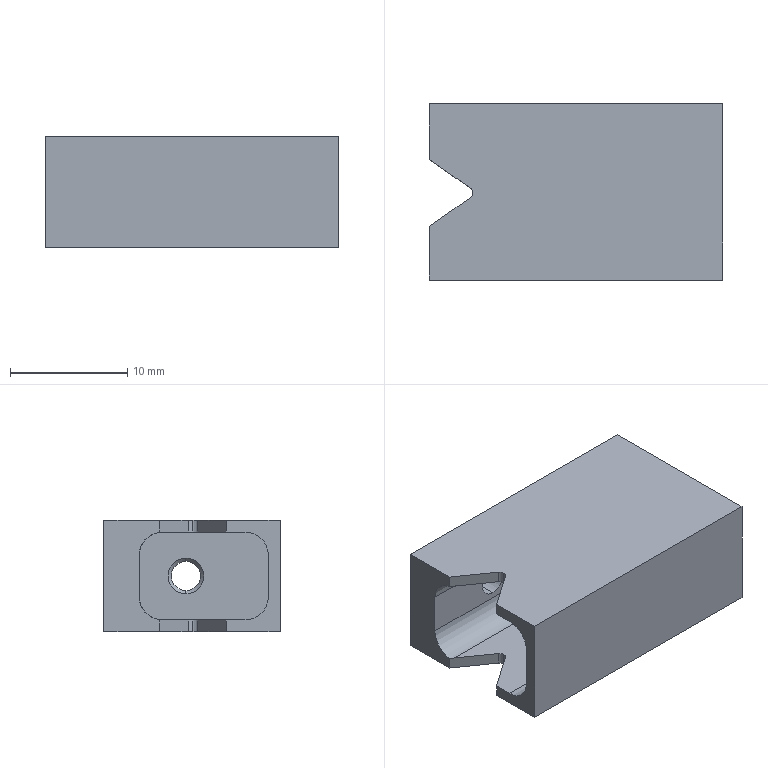Part | SolidWorks | features BaseBody 1 | 1 solid | 32 faces | box 25 x 15.037 x 9.5 mm | volume 1907 mm3 | plane 16 | cylinder 14 | cone 2 | commonest cylinder face diameters 2.5 x6 1 x4 4 x4
STEP:
#1=CARTESIAN_POINT('',(-21.301,7.437,8.5));
#2=VERTEX_POINT('',#1);
#3=CARTESIAN_POINT('',(-21.514,7.847,8.5));
#4=VERTEX_POINT('',#3);
#5=CARTESIAN_POINT('',(-21.801,7.437,8.5));
#6=DIRECTION('',(0.,0.,1.));
#7=DIRECTION('',(1.,0.,0.));
#8=AXIS2_PLACEMENT_3D('',#5,#6,#7);
#9=CIRCLE('',#8,0.5);
#10=EDGE_CURVE('',#2,#4,#9,.T.);
#11=ORIENTED_EDGE('',*,*,#10,.F.);
#12=CARTESIAN_POINT('',(-21.301,7.437,9.5));
#13=VERTEX_POINT('',#12);
#14=CARTESIAN_POINT('',(-21.301,7.437,9.5));
#15=DIRECTION('',(0.,0.,1.));
#16=VECTOR('',#15,1000.);
#17=LINE('',#14,#16);
#18=EDGE_CURVE('',#2,#13,#17,.T.);
#19=ORIENTED_EDGE('',*,*,#18,.T.);
#20=CARTESIAN_POINT('',(-21.514,7.847,9.5));
#21=VERTEX_POINT('',#20);
#22=CARTESIAN_POINT('',(-21.801,7.437,9.5));
#23=DIRECTION('',(0.,0.,1.));
#24=DIRECTION('',(1.,0.,0.));
#25=AXIS2_PLACEMENT_3D('',#22,#23,#24);
#26=CIRCLE('',#25,0.5);
#27=EDGE_CURVE('',#13,#21,#26,.T.);
#28=ORIENTED_EDGE('',*,*,#27,.T.);
#29=CARTESIAN_POINT('',(-21.514,7.847,9.5));
#30=DIRECTION('',(0.,0.,-1.));
#31=VECTOR('',#30,1000.);
#32=LINE('',#29,#31);
#33=EDGE_CURVE('',#21,#4,#32,.T.);
#34=ORIENTED_EDGE('',*,*,#33,.T.);
#35=EDGE_LOOP('',(#11,#19,#28,#34));
#36=FACE_OUTER_BOUND('',#35,.T.);
#37=CARTESIAN_POINT('',(-21.801,7.437,9.5));
#38=DIRECTION('',(0.,0.,1.));
#39=DIRECTION('',(1.,0.,0.));
#40=AXIS2_PLACEMENT_3D('',#37,#38,#39);
#41=CYLINDRICAL_SURFACE('',#40,0.5);
#42=ADVANCED_FACE('',(#36),#41,.F.);
#43=CARTESIAN_POINT('',(0.,8.037,6.));
#44=VERTEX_POINT('',#43);
#45=CARTESIAN_POINT('',(0.,8.037,3.5));
#46=VERTEX_POINT('',#45);
#47=CARTESIAN_POINT('',(0.,8.037,4.75));
#48=DIRECTION('',(1.,0.,0.));
#49=DIRECTION('',(0.,0.,1.));
#50=AXIS2_PLACEMENT_3D('',#47,#48,#49);
#51=CIRCLE('',#50,1.25);
#52=EDGE_CURVE('',#44,#46,#51,.T.);
#53=ORIENTED_EDGE('',*,*,#52,.T.);
#54=CARTESIAN_POINT('',(-4.725,8.037,3.5));
#55=VERTEX_POINT('',#54);
#56=CARTESIAN_POINT('',(-5.,8.037,3.5));
#57=DIRECTION('',(-1.,0.,0.));
#58=VECTOR('',#57,1000.);
#59=LINE('',#56,#58);
#60=EDGE_CURVE('',#46,#55,#59,.T.);
#61=ORIENTED_EDGE('',*,*,#60,.T.);
#62=CARTESIAN_POINT('',(-4.725,8.037,6.));
#63=VERTEX_POINT('',#62);
#64=CARTESIAN_POINT('',(-4.725,8.037,4.75));
#65=DIRECTION('',(1.,0.,0.));
#66=DIRECTION('',(0.,0.,1.));
#67=AXIS2_PLACEMENT_3D('',#64,#65,#66);
#68=CIRCLE('',#67,1.25);
#69=EDGE_CURVE('',#63,#55,#68,.T.);
#70=ORIENTED_EDGE('',*,*,#69,.F.);
#71=CARTESIAN_POINT('',(-5.,8.037,6.));
#72=DIRECTION('',(-1.,0.,0.));
#73=VECTOR('',#72,1000.);
#74=LINE('',#71,#73);
#75=EDGE_CURVE('',#44,#63,#74,.T.);
#76=ORIENTED_EDGE('',*,*,#75,.F.);
#77=EDGE_LOOP('',(#53,#61,#70,#76));
#78=FACE_OUTER_BOUND('',#77,.T.);
#79=CARTESIAN_POINT('',(-5.,8.037,4.75));
#80=DIRECTION('',(-1.,0.,0.));
#81=DIRECTION('',(0.,0.,1.));
#82=AXIS2_PLACEMENT_3D('',#79,#80,#81);
#83=CYLINDRICAL_SURFACE('',#82,1.25);
#84=ADVANCED_FACE('',(#78),#83,.F.);
#85=CARTESIAN_POINT('',(-18.,12.037,6.));
#86=VERTEX_POINT('',#85);
#87=CARTESIAN_POINT('',(-18.,12.037,3.5));
#88=VERTEX_POINT('',#87);
#89=CARTESIAN_POINT('',(-18.,12.037,4.75));
#90=DIRECTION('',(0.,-1.,0.));
#91=DIRECTION('',(0.,0.,1.));
#92=AXIS2_PLACEMENT_3D('',#89,#90,#91);
#93=CIRCLE('',#92,1.25);
#94=EDGE_CURVE('',#86,#88,#93,.T.);
#95=ORIENTED_EDGE('',*,*,#94,.T.);
#96=CARTESIAN_POINT('',(-18.,15.037,3.5));
#97=VERTEX_POINT('',#96);
#98=CARTESIAN_POINT('',(-18.,15.037,3.5));
#99=DIRECTION('',(0.,1.,0.));
#100=VECTOR('',#99,1000.);
#101=LINE('',#98,#100);
#102=EDGE_CURVE('',#88,#97,#101,.T.);
#103=ORIENTED_EDGE('',*,*,#102,.T.);
#104=CARTESIAN_POINT('',(-18.,15.037,6.));
#105=VERTEX_POINT('',#104);
#106=CARTESIAN_POINT('',(-18.,15.037,4.75));
#107=DIRECTION('',(0.,1.,0.));
#108=DIRECTION('',(0.,0.,1.));
#109=AXIS2_PLACEMENT_3D('',#106,#107,#108);
#110=CIRCLE('',#109,1.25);
#111=EDGE_CURVE('',#97,#105,#110,.T.);
#112=ORIENTED_EDGE('',*,*,#111,.T.);
#113=CARTESIAN_POINT('',(-18.,15.037,6.));
#114=DIRECTION('',(0.,1.,0.));
#115=VECTOR('',#114,1000.);
#116=LINE('',#113,#115);
#117=EDGE_CURVE('',#86,#105,#116,.T.);
#118=ORIENTED_EDGE('',*,*,#117,.F.);
#119=EDGE_LOOP('',(#95,#103,#112,#118));
#120=FACE_OUTER_BOUND('',#119,.T.);
#121=CARTESIAN_POINT('',(-18.,15.037,4.75));
#122=DIRECTION('',(0.,1.,0.));
#123=DIRECTION('',(0.,0.,1.));
#124=AXIS2_PLACEMENT_3D('',#121,#122,#123);
#125=CYLINDRICAL_SURFACE('',#124,1.25);
#126=ADVANCED_FACE('',(#120),#125,.F.);
#127=CARTESIAN_POINT('',(-8.,12.037,6.));
#128=VERTEX_POINT('',#127);
#129=CARTESIAN_POINT('',(-8.,12.037,3.5));
#130=VERTEX_POINT('',#129);
#131=CARTESIAN_POINT('',(-8.,12.037,4.75));
#132=DIRECTION('',(0.,-1.,0.));
#133=DIRECTION('',(0.,0.,1.));
#134=AXIS2_PLACEMENT_3D('',#131,#132,#133);
#135=CIRCLE('',#134,1.25);
#136=EDGE_CURVE('',#128,#130,#135,.T.);
#137=ORIENTED_EDGE('',*,*,#136,.T.);
#138=CARTESIAN_POINT('',(-8.,15.037,3.5));
#139=VERTEX_POINT('',#138);
#140=CARTESIAN_POINT('',(-8.,15.037,3.5));
#141=DIRECTION('',(0.,1.,0.));
#142=VECTOR('',#141,1000.);
#143=LINE('',#140,#142);
#144=EDGE_CURVE('',#130,#139,#143,.T.);
#145=ORIENTED_EDGE('',*,*,#144,.T.);
#146=CARTESIAN_POINT('',(-8.,15.037,6.));
#147=VERTEX_POINT('',#146);
#148=CARTESIAN_POINT('',(-8.,15.037,4.75));
#149=DIRECTION('',(0.,1.,0.));
#150=DIRECTION('',(0.,0.,1.));
#151=AXIS2_PLACEMENT_3D('',#148,#149,#150);
#152=CIRCLE('',#151,1.25);
#153=EDGE_CURVE('',#139,#147,#152,.T.);
#154=ORIENTED_EDGE('',*,*,#153,.T.);
#155=CARTESIAN_POINT('',(-8.,15.037,6.));
#156=DIRECTION('',(0.,1.,0.));
#157=VECTOR('',#156,1000.);
#158=LINE('',#155,#157);
#159=EDGE_CURVE('',#128,#147,#158,.T.);
#160=ORIENTED_EDGE('',*,*,#159,.F.);
#161=EDGE_LOOP('',(#137,#145,#154,#160));
#162=FACE_OUTER_BOUND('',#161,.T.);
#163=CARTESIAN_POINT('',(-8.,15.037,4.75));
#164=DIRECTION('',(0.,1.,0.));
#165=DIRECTION('',(0.,0.,1.));
#166=AXIS2_PLACEMENT_3D('',#163,#164,#165);
#167=CYLINDRICAL_SURFACE('',#166,1.25);
#168=ADVANCED_FACE('',(#162),#167,.F.);
#169=CARTESIAN_POINT('',(-21.301,7.437,0.));
#170=VERTEX_POINT('',#169);
#171=CARTESIAN_POINT('',(-21.514,7.847,0.));
#172=VERTEX_POINT('',#171);
#173=CARTESIAN_POINT('',(-21.801,7.437,0.));
#174=DIRECTION('',(0.,0.,1.));
#175=DIRECTION('',(1.,0.,0.));
#176=AXIS2_PLACEMENT_3D('',#173,#174,#175);
#177=CIRCLE('',#176,0.5);
#178=EDGE_CURVE('',#170,#172,#177,.T.);
#179=ORIENTED_EDGE('',*,*,#178,.F.);
#180=CARTESIAN_POINT('',(-21.301,7.437,1.));
#181=VERTEX_POINT('',#180);
#182=CARTESIAN_POINT('',(-21.301,7.437,9.5));
#183=DIRECTION('',(0.,0.,1.));
#184=VECTOR('',#183,1000.);
#185=LINE('',#182,#184);
#186=EDGE_CURVE('',#170,#181,#185,.T.);
#187=ORIENTED_EDGE('',*,*,#186,.T.);
#188=CARTESIAN_POINT('',(-21.514,7.847,1.));
#189=VERTEX_POINT('',#188);
#190=CARTESIAN_POINT('',(-21.801,7.437,1.));
#191=DIRECTION('',(0.,0.,1.));
#192=DIRECTION('',(1.,0.,0.));
#193=AXIS2_PLACEMENT_3D('',#190,#191,#192);
#194=CIRCLE('',#193,0.5);
#195=EDGE_CURVE('',#181,#189,#194,.T.);
#196=ORIENTED_EDGE('',*,*,#195,.T.);
#197=CARTESIAN_POINT('',(-21.514,7.847,9.5));
#198=DIRECTION('',(0.,0.,-1.));
#199=VECTOR('',#198,1000.);
#200=LINE('',#197,#199);
#201=EDGE_CURVE('',#189,#172,#200,.T.);
#202=ORIENTED_EDGE('',*,*,#201,.T.);
#203=EDGE_LOOP('',(#179,#187,#196,#202));
#204=FACE_OUTER_BOUND('',#203,.T.);
#205=CARTESIAN_POINT('',(-21.801,7.437,9.5));
#206=DIRECTION('',(0.,0.,1.));
#207=DIRECTION('',(1.,0.,0.));
#208=AXIS2_PLACEMENT_3D('',#205,#206,#207);
#209=CYLINDRICAL_SURFACE('',#208,0.5);
#210=ADVANCED_FACE('',(#204),#209,.F.);
#211=ORIENTED_EDGE('',*,*,#69,.T.);
#212=CARTESIAN_POINT('',(-5.,8.037,3.225));
#213=VERTEX_POINT('',#212);
#214=CARTESIAN_POINT('',(-5.,8.037,3.225));
#215=DIRECTION('',(-0.7071,0.,-0.7071));
#216=VECTOR('',#215,1000.);
#217=LINE('',#214,#216);
#218=EDGE_CURVE('',#55,#213,#217,.T.);
#219=ORIENTED_EDGE('',*,*,#218,.T.);
#220=CARTESIAN_POINT('',(-5.,8.037,6.275));
#221=VERTEX_POINT('',#220);
#222=CARTESIAN_POINT('',(-5.,8.037,4.75));
#223=DIRECTION('',(1.,0.,0.));
#224=DIRECTION('',(0.,0.,1.));
#225=AXIS2_PLACEMENT_3D('',#222,#223,#224);
#226=CIRCLE('',#225,1.525);
#227=EDGE_CURVE('',#221,#213,#226,.T.);
#228=ORIENTED_EDGE('',*,*,#227,.F.);
#229=CARTESIAN_POINT('',(-5.,8.037,6.275));
#230=DIRECTION('',(-0.7071,0.,0.7071));
#231=VECTOR('',#230,1000.);
#232=LINE('',#229,#231);
#233=EDGE_CURVE('',#63,#221,#232,.T.);
#234=ORIENTED_EDGE('',*,*,#233,.F.);
#235=EDGE_LOOP('',(#211,#219,#228,#234));
#236=FACE_OUTER_BOUND('',#235,.T.);
#237=CARTESIAN_POINT('',(-5.,8.037,4.75));
#238=DIRECTION('',(-1.,0.,0.));
#239=DIRECTION('',(0.,0.,1.));
#240=AXIS2_PLACEMENT_3D('',#237,#238,#239);
#241=CONICAL_SURFACE('',#240,1.525,0.7854);
#242=ADVANCED_FACE('',(#236),#241,.F.);
#243=CARTESIAN_POINT('',(-25.,10.288,9.5));
#244=VERTEX_POINT('',#243);
#245=CARTESIAN_POINT('',(-21.514,7.847,9.5));
#246=DIRECTION('',(-0.8192,0.5736,0.));
#247=VECTOR('',#246,1000.);
#248=LINE('',#245,#247);
#249=EDGE_CURVE('',#21,#244,#248,.T.);
#250=ORIENTED_EDGE('',*,*,#249,.F.);
#251=ORIENTED_EDGE('',*,*,#27,.F.);
#252=CARTESIAN_POINT('',(-21.514,7.028,9.5));
#253=VERTEX_POINT('',#252);
#254=CARTESIAN_POINT('',(-21.801,7.437,9.5));
#255=DIRECTION('',(0.,0.,1.));
#256=DIRECTION('',(1.,0.,0.));
#257=AXIS2_PLACEMENT_3D('',#254,#255,#256);
#258=CIRCLE('',#257,0.5);
#259=EDGE_CURVE('',#253,#13,#258,.T.);
#260=ORIENTED_EDGE('',*,*,#259,.F.);
#261=CARTESIAN_POINT('',(-25.,4.587,9.5));
#262=VERTEX_POINT('',#261);
#263=CARTESIAN_POINT('',(-25.,4.587,9.5));
#264=DIRECTION('',(0.8192,0.5736,0.));
#265=VECTOR('',#264,1000.);
#266=LINE('',#263,#265);
#267=EDGE_CURVE('',#262,#253,#266,.T.);
#268=ORIENTED_EDGE('',*,*,#267,.F.);
#269=CARTESIAN_POINT('',(-25.,0.,9.5));
#270=VERTEX_POINT('',#269);
#271=CARTESIAN_POINT('',(-25.,0.,9.5));
#272=DIRECTION('',(0.,1.,0.));
#273=VECTOR('',#272,1000.);
#274=LINE('',#271,#273);
#275=EDGE_CURVE('',#270,#262,#274,.T.);
#276=ORIENTED_EDGE('',*,*,#275,.F.);
#277=CARTESIAN_POINT('',(0.,0.,9.5));
#278=VERTEX_POINT('',#277);
#279=CARTESIAN_POINT('',(0.,0.,9.5));
#280=DIRECTION('',(-1.,0.,0.));
#281=VECTOR('',#280,1000.);
#282=LINE('',#279,#281);
#283=EDGE_CURVE('',#278,#270,#282,.T.);
#284=ORIENTED_EDGE('',*,*,#283,.F.);
#285=CARTESIAN_POINT('',(0.,15.037,9.5));
#286=VERTEX_POINT('',#285);
#287=CARTESIAN_POINT('',(0.,0.,9.5));
#288=DIRECTION('',(0.,-1.,0.));
#289=VECTOR('',#288,1000.);
#290=LINE('',#287,#289);
#291=EDGE_CURVE('',#286,#278,#290,.T.);
#292=ORIENTED_EDGE('',*,*,#291,.F.);
#293=CARTESIAN_POINT('',(-25.,15.037,9.5));
#294=VERTEX_POINT('',#293);
#295=CARTESIAN_POINT('',(0.,15.037,9.5));
#296=DIRECTION('',(1.,0.,0.));
#297=VECTOR('',#296,1000.);
#298=LINE('',#295,#297);
#299=EDGE_CURVE('',#294,#286,#298,.T.);
#300=ORIENTED_EDGE('',*,*,#299,.F.);
#301=CARTESIAN_POINT('',(-25.,0.,9.5));
#302=DIRECTION('',(0.,1.,0.));
#303=VECTOR('',#302,1000.);
#304=LINE('',#301,#303);
#305=EDGE_CURVE('',#244,#294,#304,.T.);
#306=ORIENTED_EDGE('',*,*,#305,.F.);
#307=EDGE_LOOP('',(#250,#251,#260,#268,#276,#284,#292,#300,#306));
#308=FACE_OUTER_BOUND('',#307,.T.);
#309=CARTESIAN_POINT('',(0.,0.,9.5));
#310=DIRECTION('',(0.,0.,-1.));
#311=DIRECTION('',(-1.,0.,0.));
#312=AXIS2_PLACEMENT_3D('',#309,#310,#311);
#313=PLANE('',#312);
#314=ADVANCED_FACE('',(#308),#313,.F.);
#315=CARTESIAN_POINT('',(-25.,12.037,3.));
#316=VERTEX_POINT('',#315);
#317=CARTESIAN_POINT('',(-25.,10.288,1.016));
#318=VERTEX_POINT('',#317);
#319=CARTESIAN_POINT('',(-25.,10.037,3.));
#320=DIRECTION('',(-1.,0.,0.));
#321=DIRECTION('',(0.,0.,-1.));
#322=AXIS2_PLACEMENT_3D('',#319,#320,#321);
#323=CIRCLE('',#322,2.);
#324=EDGE_CURVE('',#316,#318,#323,.T.);
#325=ORIENTED_EDGE('',*,*,#324,.F.);
#326=CARTESIAN_POINT('',(-25.,12.037,6.5));
#327=VERTEX_POINT('',#326);
#328=CARTESIAN_POINT('',(-25.,12.037,9.5));
#329=DIRECTION('',(0.,0.,-1.));
#330=VECTOR('',#329,1000.);
#331=LINE('',#328,#330);
#332=EDGE_CURVE('',#327,#316,#331,.T.);
#333=ORIENTED_EDGE('',*,*,#332,.F.);
#334=CARTESIAN_POINT('',(-25.,10.288,8.484));
#335=VERTEX_POINT('',#334);
#336=CARTESIAN_POINT('',(-25.,10.037,6.5));
#337=DIRECTION('',(-1.,0.,0.));
#338=DIRECTION('',(0.,0.,-1.));
#339=AXIS2_PLACEMENT_3D('',#336,#337,#338);
#340=CIRCLE('',#339,2.);
#341=EDGE_CURVE('',#335,#327,#340,.T.);
#342=ORIENTED_EDGE('',*,*,#341,.F.);
#343=CARTESIAN_POINT('',(-25.,10.288,9.5));
#344=DIRECTION('',(0.,0.,-1.));
#345=VECTOR('',#344,1000.);
#346=LINE('',#343,#345);
#347=EDGE_CURVE('',#244,#335,#346,.T.);
#348=ORIENTED_EDGE('',*,*,#347,.F.);
#349=ORIENTED_EDGE('',*,*,#305,.T.);
#350=CARTESIAN_POINT('',(-25.,15.037,0.));
#351=VERTEX_POINT('',#350);
#352=CARTESIAN_POINT('',(-25.,15.037,9.5));
#353=DIRECTION('',(0.,0.,1.));
#354=VECTOR('',#353,1000.);
#355=LINE('',#352,#354);
#356=EDGE_CURVE('',#351,#294,#355,.T.);
#357=ORIENTED_EDGE('',*,*,#356,.F.);
#358=CARTESIAN_POINT('',(-25.,10.288,0.));
#359=VERTEX_POINT('',#358);
#360=CARTESIAN_POINT('',(-25.,10.288,0.));
#361=DIRECTION('',(0.,1.,0.));
#362=VECTOR('',#361,1000.);
#363=LINE('',#360,#362);
#364=EDGE_CURVE('',#359,#351,#363,.T.);
#365=ORIENTED_EDGE('',*,*,#364,.F.);
#366=CARTESIAN_POINT('',(-25.,10.288,9.5));
#367=DIRECTION('',(0.,0.,1.));
#368=VECTOR('',#367,1000.);
#369=LINE('',#366,#368);
#370=EDGE_CURVE('',#359,#318,#369,.T.);
#371=ORIENTED_EDGE('',*,*,#370,.T.);
#372=EDGE_LOOP('',(#325,#333,#342,#348,#349,#357,#365,#371));
#373=FACE_OUTER_BOUND('',#372,.T.);
#374=CARTESIAN_POINT('',(-25.,10.288,9.5));
#375=DIRECTION('',(1.,0.,0.));
#376=DIRECTION('',(0.,0.,-1.));
#377=AXIS2_PLACEMENT_3D('',#374,#375,#376);
#378=PLANE('',#377);
#379=ADVANCED_FACE('',(#373),#378,.F.);
#380=CARTESIAN_POINT('',(-24.642,10.037,8.5));
#381=VERTEX_POINT('',#380);
#382=CARTESIAN_POINT('',(-24.642,10.037,8.5));
#383=CARTESIAN_POINT('',(-24.762,10.121,8.5));
#384=CARTESIAN_POINT('',(-24.881,10.205,8.495));
#385=CARTESIAN_POINT('',(-25.,10.288,8.484));
#386=(BOUNDED_CURVE()B_SPLINE_CURVE(3,(#382,#383,#384,#385),.UNSPECIFIED.,.F.,.F.)B_SPLINE_CURVE_WITH_KNOTS((4,4),(1.571,1.696),.UNSPECIFIED.)CURVE()GEOMETRIC_REPRESENTATION_ITEM()RATIONAL_B_SPLINE_CURVE((1.,0.9987,0.9987,1.))REPRESENTATION_ITEM(''));
#387=EDGE_CURVE('',#381,#335,#386,.T.);
#388=ORIENTED_EDGE('',*,*,#387,.F.);
#389=CARTESIAN_POINT('',(-25.,10.288,8.5));
#390=DIRECTION('',(-0.8192,0.5736,0.));
#391=VECTOR('',#390,1000.);
#392=LINE('',#389,#391);
#393=EDGE_CURVE('',#4,#381,#392,.T.);
#394=ORIENTED_EDGE('',*,*,#393,.F.);
#395=ORIENTED_EDGE('',*,*,#33,.F.);
#396=ORIENTED_EDGE('',*,*,#249,.T.);
#397=ORIENTED_EDGE('',*,*,#347,.T.);
#398=EDGE_LOOP('',(#388,#394,#395,#396,#397));
#399=FACE_OUTER_BOUND('',#398,.T.);
#400=CARTESIAN_POINT('',(-25.,10.288,9.5));
#401=DIRECTION('',(0.5736,0.8192,0.));
#402=DIRECTION('',(-0.8192,0.5736,0.));
#403=AXIS2_PLACEMENT_3D('',#400,#401,#402);
#404=PLANE('',#403);
#405=ADVANCED_FACE('',(#399),#404,.F.);
#406=ORIENTED_EDGE('',*,*,#18,.F.);
#407=CARTESIAN_POINT('',(-21.514,7.028,8.5));
#408=VERTEX_POINT('',#407);
#409=CARTESIAN_POINT('',(-21.801,7.437,8.5));
#410=DIRECTION('',(0.,0.,1.));
#411=DIRECTION('',(1.,0.,0.));
#412=AXIS2_PLACEMENT_3D('',#409,#410,#411);
#413=CIRCLE('',#412,0.5);
#414=EDGE_CURVE('',#408,#2,#413,.T.);
#415=ORIENTED_EDGE('',*,*,#414,.F.);
#416=CARTESIAN_POINT('',(-21.514,7.028,9.5));
#417=DIRECTION('',(0.,0.,-1.));
#418=VECTOR('',#417,1000.);
#419=LINE('',#416,#418);
#420=EDGE_CURVE('',#253,#408,#419,.T.);
#421=ORIENTED_EDGE('',*,*,#420,.F.);
#422=ORIENTED_EDGE('',*,*,#259,.T.);
#423=EDGE_LOOP('',(#406,#415,#421,#422));
#424=FACE_OUTER_BOUND('',#423,.T.);
#425=CARTESIAN_POINT('',(-21.801,7.437,9.5));
#426=DIRECTION('',(0.,0.,1.));
#427=DIRECTION('',(1.,0.,0.));
#428=AXIS2_PLACEMENT_3D('',#425,#426,#427);
#429=CYLINDRICAL_SURFACE('',#428,0.5);
#430=ADVANCED_FACE('',(#424),#429,.F.);
#431=ORIENTED_EDGE('',*,*,#420,.T.);
#432=CARTESIAN_POINT('',(-25.,4.587,8.5));
#433=VERTEX_POINT('',#432);
#434=CARTESIAN_POINT('',(-20.929,7.437,8.5));
#435=DIRECTION('',(0.8192,0.5736,0.));
#436=VECTOR('',#435,1000.);
#437=LINE('',#434,#436);
#438=EDGE_CURVE('',#433,#408,#437,.T.);
#439=ORIENTED_EDGE('',*,*,#438,.F.);
#440=CARTESIAN_POINT('',(-25.,4.587,9.5));
#441=DIRECTION('',(0.,0.,-1.));
#442=VECTOR('',#441,1000.);
#443=LINE('',#440,#442);
#444=EDGE_CURVE('',#262,#433,#443,.T.);
#445=ORIENTED_EDGE('',*,*,#444,.F.);
#446=ORIENTED_EDGE('',*,*,#267,.T.);
#447=EDGE_LOOP('',(#431,#439,#445,#446));
#448=FACE_OUTER_BOUND('',#447,.T.);
#449=CARTESIAN_POINT('',(-20.929,7.437,9.5));
#450=DIRECTION('',(0.5736,-0.8192,0.));
#451=DIRECTION('',(0.8192,0.5736,0.));
#452=AXIS2_PLACEMENT_3D('',#449,#450,#451);
#453=PLANE('',#452);
#454=ADVANCED_FACE('',(#448),#453,.F.);
#455=CARTESIAN_POINT('',(-25.,3.,1.));
#456=VERTEX_POINT('',#455);
#457=CARTESIAN_POINT('',(-25.,1.,3.));
#458=VERTEX_POINT('',#457);
#459=CARTESIAN_POINT('',(-25.,3.,3.));
#460=DIRECTION('',(-1.,0.,0.));
#461=DIRECTION('',(0.,0.,-1.));
#462=AXIS2_PLACEMENT_3D('',#459,#460,#461);
#463=CIRCLE('',#462,2.);
#464=EDGE_CURVE('',#456,#458,#463,.T.);
#465=ORIENTED_EDGE('',*,*,#464,.F.);
#466=CARTESIAN_POINT('',(-25.,4.587,1.));
#467=VERTEX_POINT('',#466);
#468=CARTESIAN_POINT('',(-25.,12.037,1.));
#469=DIRECTION('',(0.,1.,0.));
#470=VECTOR('',#469,1000.);
#471=LINE('',#468,#470);
#472=EDGE_CURVE('',#456,#467,#471,.T.);
#473=ORIENTED_EDGE('',*,*,#472,.T.);
#474=CARTESIAN_POINT('',(-25.,4.587,0.));
#475=VERTEX_POINT('',#474);
#476=CARTESIAN_POINT('',(-25.,4.587,9.5));
#477=DIRECTION('',(0.,0.,-1.));
#478=VECTOR('',#477,1000.);
#479=LINE('',#476,#478);
#480=EDGE_CURVE('',#467,#475,#479,.T.);
#481=ORIENTED_EDGE('',*,*,#480,.T.);
#482=CARTESIAN_POINT('',(-25.,0.,0.));
#483=VERTEX_POINT('',#482);
#484=CARTESIAN_POINT('',(-25.,4.587,0.));
#485=DIRECTION('',(0.,1.,0.));
#486=VECTOR('',#485,1000.);
#487=LINE('',#484,#486);
#488=EDGE_CURVE('',#483,#475,#487,.T.);
#489=ORIENTED_EDGE('',*,*,#488,.F.);
#490=CARTESIAN_POINT('',(-25.,0.,9.5));
#491=DIRECTION('',(0.,0.,-1.));
#492=VECTOR('',#491,1000.);
#493=LINE('',#490,#492);
#494=EDGE_CURVE('',#270,#483,#493,.T.);
#495=ORIENTED_EDGE('',*,*,#494,.F.);
#496=ORIENTED_EDGE('',*,*,#275,.T.);
#497=ORIENTED_EDGE('',*,*,#444,.T.);
#498=CARTESIAN_POINT('',(-25.,3.,8.5));
#499=VERTEX_POINT('',#498);
#500=CARTESIAN_POINT('',(-25.,4.587,8.5));
#501=DIRECTION('',(0.,1.,0.));
#502=VECTOR('',#501,1000.);
#503=LINE('',#500,#502);
#504=EDGE_CURVE('',#499,#433,#503,.T.);
#505=ORIENTED_EDGE('',*,*,#504,.F.);
#506=CARTESIAN_POINT('',(-25.,1.,6.5));
#507=VERTEX_POINT('',#506);
#508=CARTESIAN_POINT('',(-25.,3.,6.5));
#509=DIRECTION('',(-1.,0.,0.));
#510=DIRECTION('',(0.,0.,-1.));
#511=AXIS2_PLACEMENT_3D('',#508,#509,#510);
#512=CIRCLE('',#511,2.);
#513=EDGE_CURVE('',#507,#499,#512,.T.);
#514=ORIENTED_EDGE('',*,*,#513,.F.);
#515=CARTESIAN_POINT('',(-25.,1.,9.5));
#516=DIRECTION('',(0.,0.,1.));
#517=VECTOR('',#516,1000.);
#518=LINE('',#515,#517);
#519=EDGE_CURVE('',#458,#507,#518,.T.);
#520=ORIENTED_EDGE('',*,*,#519,.F.);
#521=EDGE_LOOP('',(#465,#473,#481,#489,#495,#496,#497,#505,#514,#520));
#522=FACE_OUTER_BOUND('',#521,.T.);
#523=CARTESIAN_POINT('',(-25.,4.587,9.5));
#524=DIRECTION('',(1.,0.,0.));
#525=DIRECTION('',(0.,0.,-1.));
#526=AXIS2_PLACEMENT_3D('',#523,#524,#525);
#527=PLANE('',#526);
#528=ADVANCED_FACE('',(#522),#527,.F.);
#529=CARTESIAN_POINT('',(0.,0.,0.));
#530=VERTEX_POINT('',#529);
#531=CARTESIAN_POINT('',(0.,0.,9.5));
#532=DIRECTION('',(0.,0.,-1.));
#533=VECTOR('',#532,1000.);
#534=LINE('',#531,#533);
#535=EDGE_CURVE('',#278,#530,#534,.T.);
#536=ORIENTED_EDGE('',*,*,#535,.F.);
#537=ORIENTED_EDGE('',*,*,#283,.T.);
#538=ORIENTED_EDGE('',*,*,#494,.T.);
#539=CARTESIAN_POINT('',(-25.,0.,0.));
#540=DIRECTION('',(-1.,0.,0.));
#541=VECTOR('',#540,1000.);
#542=LINE('',#539,#541);
#543=EDGE_CURVE('',#530,#483,#542,.T.);
#544=ORIENTED_EDGE('',*,*,#543,.F.);
#545=EDGE_LOOP('',(#536,#537,#538,#544));
#546=FACE_OUTER_BOUND('',#545,.T.);
#547=CARTESIAN_POINT('',(-25.,0.,9.5));
#548=DIRECTION('',(0.,1.,0.));
#549=DIRECTION('',(0.,0.,1.));
#550=AXIS2_PLACEMENT_3D('',#547,#548,#549);
#551=PLANE('',#550);
#552=ADVANCED_FACE('',(#546),#551,.F.);
#553=CARTESIAN_POINT('',(0.,15.037,0.));
#554=VERTEX_POINT('',#553);
#555=CARTESIAN_POINT('',(0.,15.037,9.5));
#556=DIRECTION('',(0.,0.,-1.));
#557=VECTOR('',#556,1000.);
#558=LINE('',#555,#557);
#559=EDGE_CURVE('',#286,#554,#558,.T.);
#560=ORIENTED_EDGE('',*,*,#559,.F.);
#561=ORIENTED_EDGE('',*,*,#291,.T.);
#562=ORIENTED_EDGE('',*,*,#535,.T.);
#563=CARTESIAN_POINT('',(0.,15.037,0.));
#564=DIRECTION('',(0.,-1.,0.));
#565=VECTOR('',#564,1000.);
#566=LINE('',#563,#565);
#567=EDGE_CURVE('',#554,#530,#566,.T.);
#568=ORIENTED_EDGE('',*,*,#567,.F.);
#569=EDGE_LOOP('',(#560,#561,#562,#568));
#570=FACE_OUTER_BOUND('',#569,.T.);
#571=ORIENTED_EDGE('',*,*,#52,.F.);
#572=CARTESIAN_POINT('',(0.,8.037,4.75));
#573=DIRECTION('',(1.,0.,0.));
#574=DIRECTION('',(0.,0.,1.));
#575=AXIS2_PLACEMENT_3D('',#572,#573,#574);
#576=CIRCLE('',#575,1.25);
#577=EDGE_CURVE('',#46,#44,#576,.T.);
#578=ORIENTED_EDGE('',*,*,#577,.F.);
#579=EDGE_LOOP('',(#571,#578));
#580=FACE_BOUND('',#579,.T.);
#581=CARTESIAN_POINT('',(0.,15.037,9.5));
#582=DIRECTION('',(-1.,0.,0.));
#583=DIRECTION('',(0.,0.,1.));
#584=AXIS2_PLACEMENT_3D('',#581,#582,#583);
#585=PLANE('',#584);
#586=ADVANCED_FACE('',(#570,#580),#585,.F.);
#587=CARTESIAN_POINT('',(-18.,15.037,4.75));
#588=DIRECTION('',(0.,1.,0.));
#589=DIRECTION('',(0.,0.,1.));
#590=AXIS2_PLACEMENT_3D('',#587,#588,#589);
#591=CIRCLE('',#590,1.25);
#592=EDGE_CURVE('',#105,#97,#591,.T.);
#593=ORIENTED_EDGE('',*,*,#592,.F.);
#594=ORIENTED_EDGE('',*,*,#111,.F.);
#595=EDGE_LOOP('',(#593,#594));
#596=FACE_BOUND('',#595,.T.);
#597=ORIENTED_EDGE('',*,*,#356,.T.);
#598=ORIENTED_EDGE('',*,*,#299,.T.);
#599=ORIENTED_EDGE('',*,*,#559,.T.);
#600=CARTESIAN_POINT('',(-25.,15.037,0.));
#601=DIRECTION('',(1.,0.,0.));
#602=VECTOR('',#601,1000.);
#603=LINE('',#600,#602);
#604=EDGE_CURVE('',#351,#554,#603,.T.);
#605=ORIENTED_EDGE('',*,*,#604,.F.);
#606=EDGE_LOOP('',(#597,#598,#599,#605));
#607=FACE_OUTER_BOUND('',#606,.T.);
#608=CARTESIAN_POINT('',(-8.,15.037,4.75));
#609=DIRECTION('',(0.,1.,0.));
#610=DIRECTION('',(0.,0.,1.));
#611=AXIS2_PLACEMENT_3D('',#608,#609,#610);
#612=CIRCLE('',#611,1.25);
#613=EDGE_CURVE('',#147,#139,#612,.T.);
#614=ORIENTED_EDGE('',*,*,#613,.F.);
#615=ORIENTED_EDGE('',*,*,#153,.F.);
#616=EDGE_LOOP('',(#614,#615));
#617=FACE_BOUND('',#616,.T.);
#618=CARTESIAN_POINT('',(-25.,15.037,9.5));
#619=DIRECTION('',(0.,-1.,0.));
#620=DIRECTION('',(0.,0.,-1.));
#621=AXIS2_PLACEMENT_3D('',#618,#619,#620);
#622=PLANE('',#621);
#623=ADVANCED_FACE('',(#596,#607,#617),#622,.F.);
#624=CARTESIAN_POINT('',(-5.,12.037,3.));
#625=VERTEX_POINT('',#624);
#626=CARTESIAN_POINT('',(13.344,12.037,3.));
#627=DIRECTION('',(1.,0.,0.));
#628=VECTOR('',#627,1000.);
#629=LINE('',#626,#628);
#630=EDGE_CURVE('',#316,#625,#629,.T.);
#631=ORIENTED_EDGE('',*,*,#630,.F.);
#632=ORIENTED_EDGE('',*,*,#324,.T.);
#633=CARTESIAN_POINT('',(-24.642,10.037,1.));
#634=VERTEX_POINT('',#633);
#635=CARTESIAN_POINT('',(-25.,10.288,1.016));
#636=CARTESIAN_POINT('',(-24.881,10.205,1.005));
#637=CARTESIAN_POINT('',(-24.762,10.121,1.));
#638=CARTESIAN_POINT('',(-24.642,10.037,1.));
#639=(BOUNDED_CURVE()B_SPLINE_CURVE(3,(#635,#636,#637,#638),.UNSPECIFIED.,.F.,.F.)B_SPLINE_CURVE_WITH_KNOTS((4,4),(4.587,4.712),.UNSPECIFIED.)CURVE()GEOMETRIC_REPRESENTATION_ITEM()RATIONAL_B_SPLINE_CURVE((1.,0.9987,0.9987,1.))REPRESENTATION_ITEM(''));
#640=EDGE_CURVE('',#318,#634,#639,.T.);
#641=ORIENTED_EDGE('',*,*,#640,.T.);
#642=CARTESIAN_POINT('',(-5.,10.037,1.));
#643=VERTEX_POINT('',#642);
#644=CARTESIAN_POINT('',(13.344,10.037,1.));
#645=DIRECTION('',(-1.,0.,0.));
#646=VECTOR('',#645,1000.);
#647=LINE('',#644,#646);
#648=EDGE_CURVE('',#643,#634,#647,.T.);
#649=ORIENTED_EDGE('',*,*,#648,.F.);
#650=CARTESIAN_POINT('',(-5.,10.037,3.));
#651=DIRECTION('',(-1.,0.,0.));
#652=DIRECTION('',(0.,0.,-1.));
#653=AXIS2_PLACEMENT_3D('',#650,#651,#652);
#654=CIRCLE('',#653,2.);
#655=EDGE_CURVE('',#625,#643,#654,.T.);
#656=ORIENTED_EDGE('',*,*,#655,.F.);
#657=EDGE_LOOP('',(#631,#632,#641,#649,#656));
#658=FACE_OUTER_BOUND('',#657,.T.);
#659=CARTESIAN_POINT('',(13.344,10.037,3.));
#660=DIRECTION('',(1.,0.,0.));
#661=DIRECTION('',(0.,0.,-1.));
#662=AXIS2_PLACEMENT_3D('',#659,#660,#661);
#663=CYLINDRICAL_SURFACE('',#662,2.);
#664=ADVANCED_FACE('',(#658),#663,.F.);
#665=CARTESIAN_POINT('',(-5.,12.037,6.5));
#666=VERTEX_POINT('',#665);
#667=CARTESIAN_POINT('',(13.344,12.037,6.5));
#668=DIRECTION('',(1.,0.,0.));
#669=VECTOR('',#668,1000.);
#670=LINE('',#667,#669);
#671=EDGE_CURVE('',#327,#666,#670,.T.);
#672=ORIENTED_EDGE('',*,*,#671,.F.);
#673=ORIENTED_EDGE('',*,*,#332,.T.);
#674=ORIENTED_EDGE('',*,*,#630,.T.);
#675=CARTESIAN_POINT('',(-5.,12.037,1.));
#676=DIRECTION('',(0.,0.,-1.));
#677=VECTOR('',#676,1000.);
#678=LINE('',#675,#677);
#679=EDGE_CURVE('',#666,#625,#678,.T.);
#680=ORIENTED_EDGE('',*,*,#679,.F.);
#681=EDGE_LOOP('',(#672,#673,#674,#680));
#682=FACE_OUTER_BOUND('',#681,.T.);
#683=ORIENTED_EDGE('',*,*,#136,.F.);
#684=CARTESIAN_POINT('',(-8.,12.037,4.75));
#685=DIRECTION('',(0.,-1.,0.));
#686=DIRECTION('',(0.,0.,1.));
#687=AXIS2_PLACEMENT_3D('',#684,#685,#686);
#688=CIRCLE('',#687,1.25);
#689=EDGE_CURVE('',#130,#128,#688,.T.);
#690=ORIENTED_EDGE('',*,*,#689,.F.);
#691=EDGE_LOOP('',(#683,#690));
#692=FACE_BOUND('',#691,.T.);
#693=ORIENTED_EDGE('',*,*,#94,.F.);
#694=CARTESIAN_POINT('',(-18.,12.037,4.75));
#695=DIRECTION('',(0.,-1.,0.));
#696=DIRECTION('',(0.,0.,1.));
#697=AXIS2_PLACEMENT_3D('',#694,#695,#696);
#698=CIRCLE('',#697,1.25);
#699=EDGE_CURVE('',#88,#86,#698,.T.);
#700=ORIENTED_EDGE('',*,*,#699,.F.);
#701=EDGE_LOOP('',(#693,#700));
#702=FACE_BOUND('',#701,.T.);
#703=CARTESIAN_POINT('',(13.344,12.037,1.));
#704=DIRECTION('',(0.,1.,0.));
#705=DIRECTION('',(0.,0.,1.));
#706=AXIS2_PLACEMENT_3D('',#703,#704,#705);
#707=PLANE('',#706);
#708=ADVANCED_FACE('',(#682,#692,#702),#707,.F.);
#709=CARTESIAN_POINT('',(-5.,10.037,8.5));
#710=VERTEX_POINT('',#709);
#711=CARTESIAN_POINT('',(13.344,10.037,8.5));
#712=DIRECTION('',(1.,0.,0.));
#713=VECTOR('',#712,1000.);
#714=LINE('',#711,#713);
#715=EDGE_CURVE('',#381,#710,#714,.T.);
#716=ORIENTED_EDGE('',*,*,#715,.F.);
#717=ORIENTED_EDGE('',*,*,#387,.T.);
#718=ORIENTED_EDGE('',*,*,#341,.T.);
#719=ORIENTED_EDGE('',*,*,#671,.T.);
#720=CARTESIAN_POINT('',(-5.,10.037,6.5));
#721=DIRECTION('',(-1.,0.,0.));
#722=DIRECTION('',(0.,0.,-1.));
#723=AXIS2_PLACEMENT_3D('',#720,#721,#722);
#724=CIRCLE('',#723,2.);
#725=EDGE_CURVE('',#710,#666,#724,.T.);
#726=ORIENTED_EDGE('',*,*,#725,.F.);
#727=EDGE_LOOP('',(#716,#717,#718,#719,#726));
#728=FACE_OUTER_BOUND('',#727,.T.);
#729=CARTESIAN_POINT('',(13.344,10.037,6.5));
#730=DIRECTION('',(1.,0.,0.));
#731=DIRECTION('',(0.,0.,-1.));
#732=AXIS2_PLACEMENT_3D('',#729,#730,#731);
#733=CYLINDRICAL_SURFACE('',#732,2.);
#734=ADVANCED_FACE('',(#728),#733,.F.);
#735=CARTESIAN_POINT('',(-21.514,7.028,0.));
#736=VERTEX_POINT('',#735);
#737=CARTESIAN_POINT('',(-21.801,7.437,0.));
#738=DIRECTION('',(0.,0.,1.));
#739=DIRECTION('',(1.,0.,0.));
#740=AXIS2_PLACEMENT_3D('',#737,#738,#739);
#741=CIRCLE('',#740,0.5);
#742=EDGE_CURVE('',#736,#170,#741,.T.);
#743=ORIENTED_EDGE('',*,*,#742,.T.);
#744=ORIENTED_EDGE('',*,*,#178,.T.);
#745=CARTESIAN_POINT('',(-21.514,7.847,0.));
#746=DIRECTION('',(-0.8192,0.5736,0.));
#747=VECTOR('',#746,1000.);
#748=LINE('',#745,#747);
#749=EDGE_CURVE('',#172,#359,#748,.T.);
#750=ORIENTED_EDGE('',*,*,#749,.T.);
#751=ORIENTED_EDGE('',*,*,#364,.T.);
#752=ORIENTED_EDGE('',*,*,#604,.T.);
#753=ORIENTED_EDGE('',*,*,#567,.T.);
#754=ORIENTED_EDGE('',*,*,#543,.T.);
#755=ORIENTED_EDGE('',*,*,#488,.T.);
#756=CARTESIAN_POINT('',(-25.,4.587,0.));
#757=DIRECTION('',(0.8192,0.5736,0.));
#758=VECTOR('',#757,1000.);
#759=LINE('',#756,#758);
#760=EDGE_CURVE('',#475,#736,#759,.T.);
#761=ORIENTED_EDGE('',*,*,#760,.T.);
#762=EDGE_LOOP('',(#743,#744,#750,#751,#752,#753,#754,#755,#761));
#763=FACE_OUTER_BOUND('',#762,.T.);
#764=CARTESIAN_POINT('',(0.,0.,0.));
#765=DIRECTION('',(0.,0.,-1.));
#766=DIRECTION('',(-1.,0.,0.));
#767=AXIS2_PLACEMENT_3D('',#764,#765,#766);
#768=PLANE('',#767);
#769=ADVANCED_FACE('',(#763),#768,.T.);
#770=CARTESIAN_POINT('',(-5.,3.,8.5));
#771=VERTEX_POINT('',#770);
#772=CARTESIAN_POINT('',(13.344,3.,8.5));
#773=DIRECTION('',(1.,0.,0.));
#774=VECTOR('',#773,1000.);
#775=LINE('',#772,#774);
#776=EDGE_CURVE('',#499,#771,#775,.T.);
#777=ORIENTED_EDGE('',*,*,#776,.F.);
#778=ORIENTED_EDGE('',*,*,#504,.T.);
#779=ORIENTED_EDGE('',*,*,#438,.T.);
#780=ORIENTED_EDGE('',*,*,#414,.T.);
#781=ORIENTED_EDGE('',*,*,#10,.T.);
#782=ORIENTED_EDGE('',*,*,#393,.T.);
#783=ORIENTED_EDGE('',*,*,#715,.T.);
#784=CARTESIAN_POINT('',(-5.,12.037,8.5));
#785=DIRECTION('',(0.,1.,0.));
#786=VECTOR('',#785,1000.);
#787=LINE('',#784,#786);
#788=EDGE_CURVE('',#771,#710,#787,.T.);
#789=ORIENTED_EDGE('',*,*,#788,.F.);
#790=EDGE_LOOP('',(#777,#778,#779,#780,#781,#782,#783,#789));
#791=FACE_OUTER_BOUND('',#790,.T.);
#792=CARTESIAN_POINT('',(13.344,12.037,8.5));
#793=DIRECTION('',(0.,0.,1.));
#794=DIRECTION('',(0.,-1.,0.));
#795=AXIS2_PLACEMENT_3D('',#792,#793,#794);
#796=PLANE('',#795);
#797=ADVANCED_FACE('',(#791),#796,.F.);
#798=CARTESIAN_POINT('',(-5.,1.,3.));
#799=VERTEX_POINT('',#798);
#800=CARTESIAN_POINT('',(13.344,1.,3.));
#801=DIRECTION('',(1.,0.,0.));
#802=VECTOR('',#801,1000.);
#803=LINE('',#800,#802);
#804=EDGE_CURVE('',#458,#799,#803,.T.);
#805=ORIENTED_EDGE('',*,*,#804,.F.);
#806=ORIENTED_EDGE('',*,*,#519,.T.);
#807=CARTESIAN_POINT('',(-5.,1.,6.5));
#808=VERTEX_POINT('',#807);
#809=CARTESIAN_POINT('',(13.344,1.,6.5));
#810=DIRECTION('',(-1.,0.,0.));
#811=VECTOR('',#810,1000.);
#812=LINE('',#809,#811);
#813=EDGE_CURVE('',#808,#507,#812,.T.);
#814=ORIENTED_EDGE('',*,*,#813,.F.);
#815=CARTESIAN_POINT('',(-5.,1.,1.));
#816=DIRECTION('',(0.,0.,1.));
#817=VECTOR('',#816,1000.);
#818=LINE('',#815,#817);
#819=EDGE_CURVE('',#799,#808,#818,.T.);
#820=ORIENTED_EDGE('',*,*,#819,.F.);
#821=EDGE_LOOP('',(#805,#806,#814,#820));
#822=FACE_OUTER_BOUND('',#821,.T.);
#823=CARTESIAN_POINT('',(13.344,1.,1.));
#824=DIRECTION('',(0.,-1.,0.));
#825=DIRECTION('',(0.,0.,-1.));
#826=AXIS2_PLACEMENT_3D('',#823,#824,#825);
#827=PLANE('',#826);
#828=ADVANCED_FACE('',(#822),#827,.F.);
#829=CARTESIAN_POINT('',(-5.,3.,1.));
#830=VERTEX_POINT('',#829);
#831=CARTESIAN_POINT('',(13.344,3.,1.));
#832=DIRECTION('',(1.,0.,0.));
#833=VECTOR('',#832,1000.);
#834=LINE('',#831,#833);
#835=EDGE_CURVE('',#456,#830,#834,.T.);
#836=ORIENTED_EDGE('',*,*,#835,.F.);
#837=ORIENTED_EDGE('',*,*,#464,.T.);
#838=ORIENTED_EDGE('',*,*,#804,.T.);
#839=CARTESIAN_POINT('',(-5.,3.,3.));
#840=DIRECTION('',(-1.,0.,0.));
#841=DIRECTION('',(0.,0.,-1.));
#842=AXIS2_PLACEMENT_3D('',#839,#840,#841);
#843=CIRCLE('',#842,2.);
#844=EDGE_CURVE('',#830,#799,#843,.T.);
#845=ORIENTED_EDGE('',*,*,#844,.F.);
#846=EDGE_LOOP('',(#836,#837,#838,#845));
#847=FACE_OUTER_BOUND('',#846,.T.);
#848=CARTESIAN_POINT('',(13.344,3.,3.));
#849=DIRECTION('',(1.,0.,0.));
#850=DIRECTION('',(0.,0.,-1.));
#851=AXIS2_PLACEMENT_3D('',#848,#849,#850);
#852=CYLINDRICAL_SURFACE('',#851,2.);
#853=ADVANCED_FACE('',(#847),#852,.F.);
#854=ORIENTED_EDGE('',*,*,#813,.T.);
#855=ORIENTED_EDGE('',*,*,#513,.T.);
#856=ORIENTED_EDGE('',*,*,#776,.T.);
#857=CARTESIAN_POINT('',(-5.,3.,6.5));
#858=DIRECTION('',(-1.,0.,0.));
#859=DIRECTION('',(0.,0.,-1.));
#860=AXIS2_PLACEMENT_3D('',#857,#858,#859);
#861=CIRCLE('',#860,2.);
#862=EDGE_CURVE('',#808,#771,#861,.T.);
#863=ORIENTED_EDGE('',*,*,#862,.F.);
#864=EDGE_LOOP('',(#854,#855,#856,#863));
#865=FACE_OUTER_BOUND('',#864,.T.);
#866=CARTESIAN_POINT('',(13.344,3.,6.5));
#867=DIRECTION('',(1.,0.,0.));
#868=DIRECTION('',(0.,0.,-1.));
#869=AXIS2_PLACEMENT_3D('',#866,#867,#868);
#870=CYLINDRICAL_SURFACE('',#869,2.);
#871=ADVANCED_FACE('',(#865),#870,.F.);
#872=ORIENTED_EDGE('',*,*,#60,.F.);
#873=ORIENTED_EDGE('',*,*,#577,.T.);
#874=ORIENTED_EDGE('',*,*,#75,.T.);
#875=CARTESIAN_POINT('',(-4.725,8.037,4.75));
#876=DIRECTION('',(1.,0.,0.));
#877=DIRECTION('',(0.,0.,1.));
#878=AXIS2_PLACEMENT_3D('',#875,#876,#877);
#879=CIRCLE('',#878,1.25);
#880=EDGE_CURVE('',#55,#63,#879,.T.);
#881=ORIENTED_EDGE('',*,*,#880,.F.);
#882=EDGE_LOOP('',(#872,#873,#874,#881));
#883=FACE_OUTER_BOUND('',#882,.T.);
#884=CARTESIAN_POINT('',(-5.,8.037,4.75));
#885=DIRECTION('',(-1.,0.,0.));
#886=DIRECTION('',(0.,0.,1.));
#887=AXIS2_PLACEMENT_3D('',#884,#885,#886);
#888=CYLINDRICAL_SURFACE('',#887,1.25);
#889=ADVANCED_FACE('',(#883),#888,.F.);
#890=ORIENTED_EDGE('',*,*,#102,.F.);
#891=ORIENTED_EDGE('',*,*,#699,.T.);
#892=ORIENTED_EDGE('',*,*,#117,.T.);
#893=ORIENTED_EDGE('',*,*,#592,.T.);
#894=EDGE_LOOP('',(#890,#891,#892,#893));
#895=FACE_OUTER_BOUND('',#894,.T.);
#896=CARTESIAN_POINT('',(-18.,15.037,4.75));
#897=DIRECTION('',(0.,1.,0.));
#898=DIRECTION('',(0.,0.,1.));
#899=AXIS2_PLACEMENT_3D('',#896,#897,#898);
#900=CYLINDRICAL_SURFACE('',#899,1.25);
#901=ADVANCED_FACE('',(#895),#900,.F.);
#902=ORIENTED_EDGE('',*,*,#144,.F.);
#903=ORIENTED_EDGE('',*,*,#689,.T.);
#904=ORIENTED_EDGE('',*,*,#159,.T.);
#905=ORIENTED_EDGE('',*,*,#613,.T.);
#906=EDGE_LOOP('',(#902,#903,#904,#905));
#907=FACE_OUTER_BOUND('',#906,.T.);
#908=CARTESIAN_POINT('',(-8.,15.037,4.75));
#909=DIRECTION('',(0.,1.,0.));
#910=DIRECTION('',(0.,0.,1.));
#911=AXIS2_PLACEMENT_3D('',#908,#909,#910);
#912=CYLINDRICAL_SURFACE('',#911,1.25);
#913=ADVANCED_FACE('',(#907),#912,.F.);
#914=ORIENTED_EDGE('',*,*,#679,.T.);
#915=ORIENTED_EDGE('',*,*,#655,.T.);
#916=CARTESIAN_POINT('',(-5.,15.037,1.));
#917=DIRECTION('',(0.,-1.,0.));
#918=VECTOR('',#917,1000.);
#919=LINE('',#916,#918);
#920=EDGE_CURVE('',#643,#830,#919,.T.);
#921=ORIENTED_EDGE('',*,*,#920,.T.);
#922=ORIENTED_EDGE('',*,*,#844,.T.);
#923=ORIENTED_EDGE('',*,*,#819,.T.);
#924=ORIENTED_EDGE('',*,*,#862,.T.);
#925=ORIENTED_EDGE('',*,*,#788,.T.);
#926=ORIENTED_EDGE('',*,*,#725,.T.);
#927=EDGE_LOOP('',(#914,#915,#921,#922,#923,#924,#925,#926));
#928=FACE_OUTER_BOUND('',#927,.T.);
#929=ORIENTED_EDGE('',*,*,#227,.T.);
#930=CARTESIAN_POINT('',(-5.,8.037,4.75));
#931=DIRECTION('',(1.,0.,0.));
#932=DIRECTION('',(0.,0.,1.));
#933=AXIS2_PLACEMENT_3D('',#930,#931,#932);
#934=CIRCLE('',#933,1.525);
#935=EDGE_CURVE('',#213,#221,#934,.T.);
#936=ORIENTED_EDGE('',*,*,#935,.T.);
#937=EDGE_LOOP('',(#929,#936));
#938=FACE_BOUND('',#937,.T.);
#939=CARTESIAN_POINT('',(-5.,15.037,9.5));
#940=DIRECTION('',(-1.,0.,0.));
#941=DIRECTION('',(0.,0.,1.));
#942=AXIS2_PLACEMENT_3D('',#939,#940,#941);
#943=PLANE('',#942);
#944=ADVANCED_FACE('',(#928,#938),#943,.T.);
#945=ORIENTED_EDGE('',*,*,#835,.T.);
#946=ORIENTED_EDGE('',*,*,#920,.F.);
#947=ORIENTED_EDGE('',*,*,#648,.T.);
#948=CARTESIAN_POINT('',(-21.514,7.847,1.));
#949=DIRECTION('',(-0.8192,0.5736,0.));
#950=VECTOR('',#949,1000.);
#951=LINE('',#948,#950);
#952=EDGE_CURVE('',#189,#634,#951,.T.);
#953=ORIENTED_EDGE('',*,*,#952,.F.);
#954=ORIENTED_EDGE('',*,*,#195,.F.);
#955=CARTESIAN_POINT('',(-21.514,7.028,1.));
#956=VERTEX_POINT('',#955);
#957=CARTESIAN_POINT('',(-21.801,7.437,1.));
#958=DIRECTION('',(0.,0.,1.));
#959=DIRECTION('',(1.,0.,0.));
#960=AXIS2_PLACEMENT_3D('',#957,#958,#959);
#961=CIRCLE('',#960,0.5);
#962=EDGE_CURVE('',#956,#181,#961,.T.);
#963=ORIENTED_EDGE('',*,*,#962,.F.);
#964=CARTESIAN_POINT('',(-25.,4.587,1.));
#965=DIRECTION('',(0.8192,0.5736,0.));
#966=VECTOR('',#965,1000.);
#967=LINE('',#964,#966);
#968=EDGE_CURVE('',#467,#956,#967,.T.);
#969=ORIENTED_EDGE('',*,*,#968,.F.);
#970=ORIENTED_EDGE('',*,*,#472,.F.);
#971=EDGE_LOOP('',(#945,#946,#947,#953,#954,#963,#969,#970));
#972=FACE_OUTER_BOUND('',#971,.T.);
#973=CARTESIAN_POINT('',(13.344,12.037,1.));
#974=DIRECTION('',(0.,0.,-1.));
#975=DIRECTION('',(0.,1.,0.));
#976=AXIS2_PLACEMENT_3D('',#973,#974,#975);
#977=PLANE('',#976);
#978=ADVANCED_FACE('',(#972),#977,.F.);
#979=ORIENTED_EDGE('',*,*,#201,.F.);
#980=ORIENTED_EDGE('',*,*,#952,.T.);
#981=ORIENTED_EDGE('',*,*,#640,.F.);
#982=ORIENTED_EDGE('',*,*,#370,.F.);
#983=ORIENTED_EDGE('',*,*,#749,.F.);
#984=EDGE_LOOP('',(#979,#980,#981,#982,#983));
#985=FACE_OUTER_BOUND('',#984,.T.);
#986=CARTESIAN_POINT('',(-25.,10.288,9.5));
#987=DIRECTION('',(0.5736,0.8192,0.));
#988=DIRECTION('',(-0.8192,0.5736,0.));
#989=AXIS2_PLACEMENT_3D('',#986,#987,#988);
#990=PLANE('',#989);
#991=ADVANCED_FACE('',(#985),#990,.F.);
#992=ORIENTED_EDGE('',*,*,#186,.F.);
#993=ORIENTED_EDGE('',*,*,#742,.F.);
#994=CARTESIAN_POINT('',(-21.514,7.028,9.5));
#995=DIRECTION('',(0.,0.,-1.));
#996=VECTOR('',#995,1000.);
#997=LINE('',#994,#996);
#998=EDGE_CURVE('',#956,#736,#997,.T.);
#999=ORIENTED_EDGE('',*,*,#998,.F.);
#1000=ORIENTED_EDGE('',*,*,#962,.T.);
#1001=EDGE_LOOP('',(#992,#993,#999,#1000));
#1002=FACE_OUTER_BOUND('',#1001,.T.);
#1003=CARTESIAN_POINT('',(-21.801,7.437,9.5));
#1004=DIRECTION('',(0.,0.,1.));
#1005=DIRECTION('',(1.,0.,0.));
#1006=AXIS2_PLACEMENT_3D('',#1003,#1004,#1005);
#1007=CYLINDRICAL_SURFACE('',#1006,0.5);
#1008=ADVANCED_FACE('',(#1002),#1007,.F.);
#1009=ORIENTED_EDGE('',*,*,#998,.T.);
#1010=ORIENTED_EDGE('',*,*,#760,.F.);
#1011=ORIENTED_EDGE('',*,*,#480,.F.);
#1012=ORIENTED_EDGE('',*,*,#968,.T.);
#1013=EDGE_LOOP('',(#1009,#1010,#1011,#1012));
#1014=FACE_OUTER_BOUND('',#1013,.T.);
#1015=CARTESIAN_POINT('',(-20.929,7.437,9.5));
#1016=DIRECTION('',(0.5736,-0.8192,0.));
#1017=DIRECTION('',(0.8192,0.5736,0.));
#1018=AXIS2_PLACEMENT_3D('',#1015,#1016,#1017);
#1019=PLANE('',#1018);
#1020=ADVANCED_FACE('',(#1014),#1019,.F.);
#1021=ORIENTED_EDGE('',*,*,#218,.F.);
#1022=ORIENTED_EDGE('',*,*,#880,.T.);
#1023=ORIENTED_EDGE('',*,*,#233,.T.);
#1024=ORIENTED_EDGE('',*,*,#935,.F.);
#1025=EDGE_LOOP('',(#1021,#1022,#1023,#1024));
#1026=FACE_OUTER_BOUND('',#1025,.T.);
#1027=CARTESIAN_POINT('',(-5.,8.037,4.75));
#1028=DIRECTION('',(-1.,0.,0.));
#1029=DIRECTION('',(0.,0.,1.));
#1030=AXIS2_PLACEMENT_3D('',#1027,#1028,#1029);
#1031=CONICAL_SURFACE('',#1030,1.525,0.7854);
#1032=ADVANCED_FACE('',(#1026),#1031,.F.);
#1033=CLOSED_SHELL('',(#42,#84,#126,#168,#210,#242,#314,#379,#405,#430,#454,#528,#552,#586,#623,#664,#708,#734,#769,#797,#828,#853,#871,#889,#901,#913,#944,#978,#991,#1008,#1020,#1032));
#1034=MANIFOLD_SOLID_BREP('',#1033);
#1035=CARTESIAN_POINT('',(0.,0.,0.));
#1036=DIRECTION('',(0.,0.,1.));
#1037=DIRECTION('',(1.,0.,0.));
#1038=AXIS2_PLACEMENT_3D('',#1035,#1036,#1037);
#1039=(LENGTH_UNIT()NAMED_UNIT(*)SI_UNIT(.MILLI.,.METRE.));
#1040=UNCERTAINTY_MEASURE_WITH_UNIT(LENGTH_MEASURE(0.00001),#1039,'','');
#1041=(NAMED_UNIT(*)PLANE_ANGLE_UNIT()SI_UNIT($,.RADIAN.));
#1042=(NAMED_UNIT(*)SI_UNIT($,.STERADIAN.)SOLID_ANGLE_UNIT());
#1043=(GEOMETRIC_REPRESENTATION_CONTEXT(3)GLOBAL_UNCERTAINTY_ASSIGNED_CONTEXT((#1040))GLOBAL_UNIT_ASSIGNED_CONTEXT((#1039,#1041,#1042))REPRESENTATION_CONTEXT('',''));
#1044=ADVANCED_BREP_SHAPE_REPRESENTATION('',(#1034,#1038),#1043);